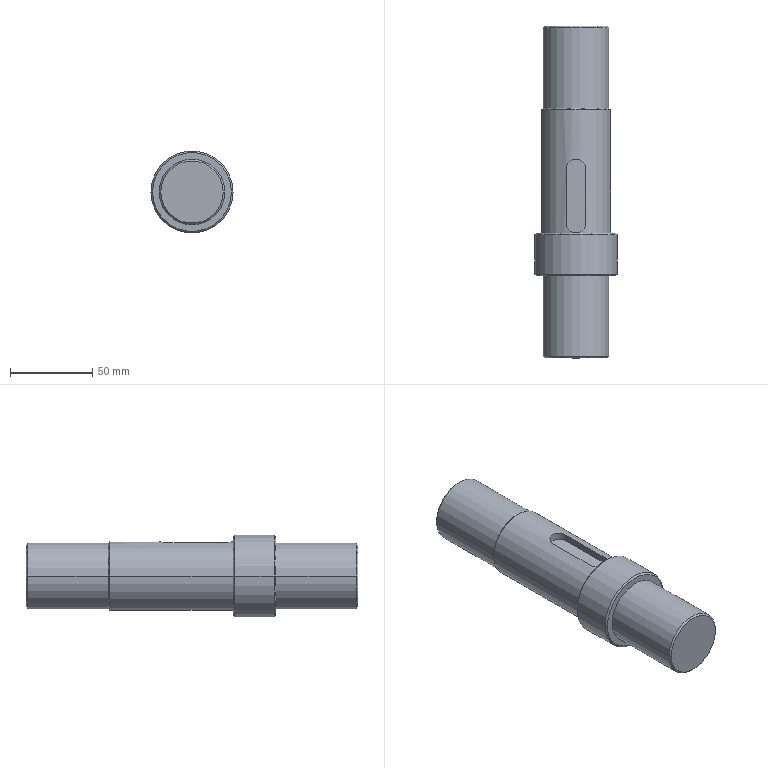Part | SolidWorks | features Chamfer 1, ICE 1, Revolution 1 | 1 solid | 27 faces | box 50 x 202 x 50 mm | volume 279258 mm3 | cone 10 | cylinder 10 | plane 7 | commonest cylinder face diameters 40 x4 12 x2 42 x2 50 x2
STEP:
#1=CARTESIAN_POINT('',(19.,0.,0.));
#2=VERTEX_POINT('',#1);
#3=CARTESIAN_POINT('',(-19.,0.,0.));
#4=VERTEX_POINT('',#3);
#5=CARTESIAN_POINT('',(0.,0.,0.));
#6=DIRECTION('',(0.,-1.,0.));
#7=DIRECTION('',(-1.,0.,0.));
#8=AXIS2_PLACEMENT_3D('',#5,#6,#7);
#9=CIRCLE('',#8,19.);
#10=EDGE_CURVE('',#2,#4,#9,.T.);
#11=ORIENTED_EDGE('',*,*,#10,.F.);
#12=CARTESIAN_POINT('',(20.,1.,0.));
#13=VERTEX_POINT('',#12);
#14=CARTESIAN_POINT('',(20.,1.,0.));
#15=DIRECTION('',(0.7071,0.7071,0.));
#16=VECTOR('',#15,1000.);
#17=LINE('',#14,#16);
#18=EDGE_CURVE('',#2,#13,#17,.T.);
#19=ORIENTED_EDGE('',*,*,#18,.T.);
#20=CARTESIAN_POINT('',(-20.,1.,0.));
#21=VERTEX_POINT('',#20);
#22=CARTESIAN_POINT('',(0.,1.,0.));
#23=DIRECTION('',(0.,1.,0.));
#24=DIRECTION('',(-1.,0.,0.));
#25=AXIS2_PLACEMENT_3D('',#22,#23,#24);
#26=CIRCLE('',#25,20.);
#27=EDGE_CURVE('',#21,#13,#26,.T.);
#28=ORIENTED_EDGE('',*,*,#27,.F.);
#29=CARTESIAN_POINT('',(-20.,1.,0.));
#30=DIRECTION('',(-0.7071,0.7071,0.));
#31=VECTOR('',#30,1000.);
#32=LINE('',#29,#31);
#33=EDGE_CURVE('',#4,#21,#32,.T.);
#34=ORIENTED_EDGE('',*,*,#33,.F.);
#35=EDGE_LOOP('',(#11,#19,#28,#34));
#36=FACE_OUTER_BOUND('',#35,.T.);
#37=CARTESIAN_POINT('',(0.,1.,0.));
#38=DIRECTION('',(0.,1.,0.));
#39=DIRECTION('',(-1.,0.,0.));
#40=AXIS2_PLACEMENT_3D('',#37,#38,#39);
#41=CONICAL_SURFACE('',#40,20.,0.7854);
#42=ADVANCED_FACE('',(#36),#41,.T.);
#43=CARTESIAN_POINT('',(-20.,152.,0.));
#44=VERTEX_POINT('',#43);
#45=CARTESIAN_POINT('',(20.,152.,0.));
#46=VERTEX_POINT('',#45);
#47=CARTESIAN_POINT('',(0.,152.,0.));
#48=DIRECTION('',(0.,1.,0.));
#49=DIRECTION('',(-1.,0.,0.));
#50=AXIS2_PLACEMENT_3D('',#47,#48,#49);
#51=CIRCLE('',#50,20.);
#52=EDGE_CURVE('',#44,#46,#51,.T.);
#53=ORIENTED_EDGE('',*,*,#52,.F.);
#54=CARTESIAN_POINT('',(-21.,151.,0.));
#55=VERTEX_POINT('',#54);
#56=CARTESIAN_POINT('',(-20.,152.,0.));
#57=DIRECTION('',(-0.7071,-0.7071,0.));
#58=VECTOR('',#57,1000.);
#59=LINE('',#56,#58);
#60=EDGE_CURVE('',#44,#55,#59,.T.);
#61=ORIENTED_EDGE('',*,*,#60,.T.);
#62=CARTESIAN_POINT('',(21.,151.,0.));
#63=VERTEX_POINT('',#62);
#64=CARTESIAN_POINT('',(0.,151.,0.));
#65=DIRECTION('',(0.,-1.,0.));
#66=DIRECTION('',(1.,0.,0.));
#67=AXIS2_PLACEMENT_3D('',#64,#65,#66);
#68=CIRCLE('',#67,21.);
#69=EDGE_CURVE('',#63,#55,#68,.T.);
#70=ORIENTED_EDGE('',*,*,#69,.F.);
#71=CARTESIAN_POINT('',(20.,152.,0.));
#72=DIRECTION('',(0.7071,-0.7071,0.));
#73=VECTOR('',#72,1000.);
#74=LINE('',#71,#73);
#75=EDGE_CURVE('',#46,#63,#74,.T.);
#76=ORIENTED_EDGE('',*,*,#75,.F.);
#77=EDGE_LOOP('',(#53,#61,#70,#76));
#78=FACE_OUTER_BOUND('',#77,.T.);
#79=CARTESIAN_POINT('',(0.,152.,0.));
#80=DIRECTION('',(0.,-1.,0.));
#81=DIRECTION('',(1.,0.,0.));
#82=AXIS2_PLACEMENT_3D('',#79,#80,#81);
#83=CONICAL_SURFACE('',#82,20.,0.7854);
#84=ADVANCED_FACE('',(#78),#83,.T.);
#85=CARTESIAN_POINT('',(-19.,202.,0.));
#86=VERTEX_POINT('',#85);
#87=CARTESIAN_POINT('',(19.,202.,0.));
#88=VERTEX_POINT('',#87);
#89=CARTESIAN_POINT('',(0.,202.,0.));
#90=DIRECTION('',(0.,1.,0.));
#91=DIRECTION('',(1.,0.,0.));
#92=AXIS2_PLACEMENT_3D('',#89,#90,#91);
#93=CIRCLE('',#92,19.);
#94=EDGE_CURVE('',#86,#88,#93,.T.);
#95=ORIENTED_EDGE('',*,*,#94,.F.);
#96=CARTESIAN_POINT('',(-20.,201.,0.));
#97=VERTEX_POINT('',#96);
#98=CARTESIAN_POINT('',(-19.,202.,0.));
#99=DIRECTION('',(-0.7071,-0.7071,0.));
#100=VECTOR('',#99,1000.);
#101=LINE('',#98,#100);
#102=EDGE_CURVE('',#86,#97,#101,.T.);
#103=ORIENTED_EDGE('',*,*,#102,.T.);
#104=CARTESIAN_POINT('',(20.,201.,0.));
#105=VERTEX_POINT('',#104);
#106=CARTESIAN_POINT('',(0.,201.,0.));
#107=DIRECTION('',(0.,-1.,0.));
#108=DIRECTION('',(1.,0.,0.));
#109=AXIS2_PLACEMENT_3D('',#106,#107,#108);
#110=CIRCLE('',#109,20.);
#111=EDGE_CURVE('',#105,#97,#110,.T.);
#112=ORIENTED_EDGE('',*,*,#111,.F.);
#113=CARTESIAN_POINT('',(19.,202.,0.));
#114=DIRECTION('',(0.7071,-0.7071,0.));
#115=VECTOR('',#114,1000.);
#116=LINE('',#113,#115);
#117=EDGE_CURVE('',#88,#105,#116,.T.);
#118=ORIENTED_EDGE('',*,*,#117,.F.);
#119=EDGE_LOOP('',(#95,#103,#112,#118));
#120=FACE_OUTER_BOUND('',#119,.T.);
#121=CARTESIAN_POINT('',(0.,202.,0.));
#122=DIRECTION('',(0.,-1.,0.));
#123=DIRECTION('',(1.,0.,0.));
#124=AXIS2_PLACEMENT_3D('',#121,#122,#123);
#125=CONICAL_SURFACE('',#124,19.,0.7854);
#126=ADVANCED_FACE('',(#120),#125,.T.);
#127=CARTESIAN_POINT('',(-24.,76.,0.));
#128=VERTEX_POINT('',#127);
#129=CARTESIAN_POINT('',(24.,76.,0.));
#130=VERTEX_POINT('',#129);
#131=CARTESIAN_POINT('',(0.,76.,0.));
#132=DIRECTION('',(0.,1.,0.));
#133=DIRECTION('',(1.,0.,0.));
#134=AXIS2_PLACEMENT_3D('',#131,#132,#133);
#135=CIRCLE('',#134,24.);
#136=EDGE_CURVE('',#128,#130,#135,.T.);
#137=ORIENTED_EDGE('',*,*,#136,.F.);
#138=CARTESIAN_POINT('',(-25.,75.,0.));
#139=VERTEX_POINT('',#138);
#140=CARTESIAN_POINT('',(-24.,76.,0.));
#141=DIRECTION('',(-0.7071,-0.7071,0.));
#142=VECTOR('',#141,1000.);
#143=LINE('',#140,#142);
#144=EDGE_CURVE('',#128,#139,#143,.T.);
#145=ORIENTED_EDGE('',*,*,#144,.T.);
#146=CARTESIAN_POINT('',(25.,75.,0.));
#147=VERTEX_POINT('',#146);
#148=CARTESIAN_POINT('',(0.,75.,0.));
#149=DIRECTION('',(0.,-1.,0.));
#150=DIRECTION('',(1.,0.,0.));
#151=AXIS2_PLACEMENT_3D('',#148,#149,#150);
#152=CIRCLE('',#151,25.);
#153=EDGE_CURVE('',#147,#139,#152,.T.);
#154=ORIENTED_EDGE('',*,*,#153,.F.);
#155=CARTESIAN_POINT('',(24.,76.,0.));
#156=DIRECTION('',(0.7071,-0.7071,0.));
#157=VECTOR('',#156,1000.);
#158=LINE('',#155,#157);
#159=EDGE_CURVE('',#130,#147,#158,.T.);
#160=ORIENTED_EDGE('',*,*,#159,.F.);
#161=EDGE_LOOP('',(#137,#145,#154,#160));
#162=FACE_OUTER_BOUND('',#161,.T.);
#163=CARTESIAN_POINT('',(0.,76.,0.));
#164=DIRECTION('',(0.,-1.,0.));
#165=DIRECTION('',(1.,0.,0.));
#166=AXIS2_PLACEMENT_3D('',#163,#164,#165);
#167=CONICAL_SURFACE('',#166,24.,0.7854);
#168=ADVANCED_FACE('',(#162),#167,.T.);
#169=CARTESIAN_POINT('',(24.,50.,0.));
#170=VERTEX_POINT('',#169);
#171=CARTESIAN_POINT('',(-24.,50.,0.));
#172=VERTEX_POINT('',#171);
#173=CARTESIAN_POINT('',(0.,50.,0.));
#174=DIRECTION('',(0.,-1.,0.));
#175=DIRECTION('',(-1.,0.,0.));
#176=AXIS2_PLACEMENT_3D('',#173,#174,#175);
#177=CIRCLE('',#176,24.);
#178=EDGE_CURVE('',#170,#172,#177,.T.);
#179=ORIENTED_EDGE('',*,*,#178,.F.);
#180=CARTESIAN_POINT('',(25.,51.,0.));
#181=VERTEX_POINT('',#180);
#182=CARTESIAN_POINT('',(25.,51.,0.));
#183=DIRECTION('',(0.7071,0.7071,0.));
#184=VECTOR('',#183,1000.);
#185=LINE('',#182,#184);
#186=EDGE_CURVE('',#170,#181,#185,.T.);
#187=ORIENTED_EDGE('',*,*,#186,.T.);
#188=CARTESIAN_POINT('',(-25.,51.,0.));
#189=VERTEX_POINT('',#188);
#190=CARTESIAN_POINT('',(0.,51.,0.));
#191=DIRECTION('',(0.,1.,0.));
#192=DIRECTION('',(-1.,0.,0.));
#193=AXIS2_PLACEMENT_3D('',#190,#191,#192);
#194=CIRCLE('',#193,25.);
#195=EDGE_CURVE('',#189,#181,#194,.T.);
#196=ORIENTED_EDGE('',*,*,#195,.F.);
#197=CARTESIAN_POINT('',(-25.,51.,0.));
#198=DIRECTION('',(-0.7071,0.7071,0.));
#199=VECTOR('',#198,1000.);
#200=LINE('',#197,#199);
#201=EDGE_CURVE('',#172,#189,#200,.T.);
#202=ORIENTED_EDGE('',*,*,#201,.F.);
#203=EDGE_LOOP('',(#179,#187,#196,#202));
#204=FACE_OUTER_BOUND('',#203,.T.);
#205=CARTESIAN_POINT('',(0.,51.,0.));
#206=DIRECTION('',(0.,1.,0.));
#207=DIRECTION('',(-1.,0.,0.));
#208=AXIS2_PLACEMENT_3D('',#205,#206,#207);
#209=CONICAL_SURFACE('',#208,25.,0.7854);
#210=ADVANCED_FACE('',(#204),#209,.T.);
#211=ORIENTED_EDGE('',*,*,#52,.T.);
#212=CARTESIAN_POINT('',(20.,202.,0.));
#213=DIRECTION('',(0.,1.,0.));
#214=VECTOR('',#213,1000.);
#215=LINE('',#212,#214);
#216=EDGE_CURVE('',#46,#105,#215,.T.);
#217=ORIENTED_EDGE('',*,*,#216,.T.);
#218=ORIENTED_EDGE('',*,*,#111,.T.);
#219=CARTESIAN_POINT('',(-20.,202.,0.));
#220=DIRECTION('',(0.,1.,0.));
#221=VECTOR('',#220,1000.);
#222=LINE('',#219,#221);
#223=EDGE_CURVE('',#44,#97,#222,.T.);
#224=ORIENTED_EDGE('',*,*,#223,.F.);
#225=EDGE_LOOP('',(#211,#217,#218,#224));
#226=FACE_OUTER_BOUND('',#225,.T.);
#227=CARTESIAN_POINT('',(0.,202.,0.));
#228=DIRECTION('',(0.,1.,0.));
#229=DIRECTION('',(-1.,0.,0.));
#230=AXIS2_PLACEMENT_3D('',#227,#228,#229);
#231=CYLINDRICAL_SURFACE('',#230,20.);
#232=ADVANCED_FACE('',(#226),#231,.T.);
#233=ORIENTED_EDGE('',*,*,#195,.T.);
#234=CARTESIAN_POINT('',(25.,202.,0.));
#235=DIRECTION('',(0.,1.,0.));
#236=VECTOR('',#235,1000.);
#237=LINE('',#234,#236);
#238=EDGE_CURVE('',#181,#147,#237,.T.);
#239=ORIENTED_EDGE('',*,*,#238,.T.);
#240=ORIENTED_EDGE('',*,*,#153,.T.);
#241=CARTESIAN_POINT('',(-25.,202.,0.));
#242=DIRECTION('',(0.,1.,0.));
#243=VECTOR('',#242,1000.);
#244=LINE('',#241,#243);
#245=EDGE_CURVE('',#189,#139,#244,.T.);
#246=ORIENTED_EDGE('',*,*,#245,.F.);
#247=EDGE_LOOP('',(#233,#239,#240,#246));
#248=FACE_OUTER_BOUND('',#247,.T.);
#249=CARTESIAN_POINT('',(0.,202.,0.));
#250=DIRECTION('',(0.,1.,0.));
#251=DIRECTION('',(-1.,0.,0.));
#252=AXIS2_PLACEMENT_3D('',#249,#250,#251);
#253=CYLINDRICAL_SURFACE('',#252,25.);
#254=ADVANCED_FACE('',(#248),#253,.T.);
#255=ORIENTED_EDGE('',*,*,#27,.T.);
#256=CARTESIAN_POINT('',(20.,50.,0.));
#257=VERTEX_POINT('',#256);
#258=CARTESIAN_POINT('',(20.,202.,0.));
#259=DIRECTION('',(0.,1.,0.));
#260=VECTOR('',#259,1000.);
#261=LINE('',#258,#260);
#262=EDGE_CURVE('',#13,#257,#261,.T.);
#263=ORIENTED_EDGE('',*,*,#262,.T.);
#264=CARTESIAN_POINT('',(-20.,50.,0.));
#265=VERTEX_POINT('',#264);
#266=CARTESIAN_POINT('',(0.,50.,0.));
#267=DIRECTION('',(0.,1.,0.));
#268=DIRECTION('',(-1.,0.,0.));
#269=AXIS2_PLACEMENT_3D('',#266,#267,#268);
#270=CIRCLE('',#269,20.);
#271=EDGE_CURVE('',#265,#257,#270,.T.);
#272=ORIENTED_EDGE('',*,*,#271,.F.);
#273=CARTESIAN_POINT('',(-20.,202.,0.));
#274=DIRECTION('',(0.,1.,0.));
#275=VECTOR('',#274,1000.);
#276=LINE('',#273,#275);
#277=EDGE_CURVE('',#21,#265,#276,.T.);
#278=ORIENTED_EDGE('',*,*,#277,.F.);
#279=EDGE_LOOP('',(#255,#263,#272,#278));
#280=FACE_OUTER_BOUND('',#279,.T.);
#281=CARTESIAN_POINT('',(0.,202.,0.));
#282=DIRECTION('',(0.,1.,0.));
#283=DIRECTION('',(-1.,0.,0.));
#284=AXIS2_PLACEMENT_3D('',#281,#282,#283);
#285=CYLINDRICAL_SURFACE('',#284,20.);
#286=ADVANCED_FACE('',(#280),#285,.T.);
#287=CARTESIAN_POINT('',(-6.,82.01,20.125));
#288=VERTEX_POINT('',#287);
#289=CARTESIAN_POINT('',(6.,82.01,20.125));
#290=VERTEX_POINT('',#289);
#291=CARTESIAN_POINT('',(-6.,82.01,20.125));
#292=CARTESIAN_POINT('',(-6.,81.611,20.125));
#293=CARTESIAN_POINT('',(-5.961,81.22,20.136));
#294=CARTESIAN_POINT('',(-5.845,80.643,20.17));
#295=CARTESIAN_POINT('',(-5.798,80.452,20.184));
#296=CARTESIAN_POINT('',(-5.683,80.074,20.217));
#297=CARTESIAN_POINT('',(-5.615,79.887,20.235));
#298=CARTESIAN_POINT('',(-5.389,79.343,20.297));
#299=CARTESIAN_POINT('',(-5.205,78.999,20.346));
#300=CARTESIAN_POINT('',(-4.878,78.512,20.426));
#301=CARTESIAN_POINT('',(-4.761,78.353,20.454));
#302=CARTESIAN_POINT('',(-4.511,78.05,20.51));
#303=CARTESIAN_POINT('',(-4.38,77.905,20.539));
#304=CARTESIAN_POINT('',(-3.968,77.492,20.624));
#305=CARTESIAN_POINT('',(-3.667,77.245,20.68));
#306=CARTESIAN_POINT('',(-3.012,76.806,20.785));
#307=CARTESIAN_POINT('',(-2.666,76.621,20.833));
#308=CARTESIAN_POINT('',(-2.126,76.396,20.893));
#309=CARTESIAN_POINT('',(-1.942,76.329,20.911));
#310=CARTESIAN_POINT('',(-1.565,76.214,20.942));
#311=CARTESIAN_POINT('',(-1.371,76.165,20.956));
#312=CARTESIAN_POINT('',(-0.7899,76.049,20.989));
#313=CARTESIAN_POINT('',(-0.3993,76.01,21.));
#314=CARTESIAN_POINT('',(0.3878,76.01,21.));
#315=CARTESIAN_POINT('',(0.7877,76.049,20.989));
#316=CARTESIAN_POINT('',(1.559,76.203,20.946));
#317=CARTESIAN_POINT('',(1.934,76.317,20.914));
#318=CARTESIAN_POINT('',(2.481,76.543,20.854));
#319=CARTESIAN_POINT('',(2.66,76.628,20.832));
#320=CARTESIAN_POINT('',(3.006,76.813,20.785));
#321=CARTESIAN_POINT('',(3.173,76.914,20.76));
#322=CARTESIAN_POINT('',(3.497,77.13,20.707));
#323=CARTESIAN_POINT('',(3.653,77.247,20.68));
#324=CARTESIAN_POINT('',(3.956,77.495,20.625));
#325=CARTESIAN_POINT('',(4.103,77.627,20.596));
#326=CARTESIAN_POINT('',(4.518,78.043,20.51));
#327=CARTESIAN_POINT('',(4.765,78.343,20.453));
#328=CARTESIAN_POINT('',(5.2,78.991,20.347));
#329=CARTESIAN_POINT('',(5.389,79.342,20.297));
#330=CARTESIAN_POINT('',(5.69,80.065,20.215));
#331=CARTESIAN_POINT('',(5.804,80.439,20.182));
#332=CARTESIAN_POINT('',(5.96,81.213,20.137));
#333=CARTESIAN_POINT('',(6.,81.611,20.125));
#334=CARTESIAN_POINT('',(6.,82.01,20.125));
#335=B_SPLINE_CURVE_WITH_KNOTS('',3,(#291,#292,#293,#294,#295,#296,#297,#298,#299,#300,#301,#302,#303,#304,#305,#306,#307,#308,#309,#310,#311,#312,#313,#314,#315,#316,#317,#318,#319,#320,#321,#322,#323,#324,#325,#326,#327,#328,#329,#330,#331,#332,#333,#334),.UNSPECIFIED.,.F.,.F.,(4,2,2,2,2,2,2,2,2,2,2,2,2,2,2,2,2,2,2,2,2,4),(0.,0.001178,0.001767,0.002356,0.003535,0.004124,0.004713,0.005891,0.007069,0.007658,0.008247,0.009425,0.0106,0.01178,0.01237,0.01296,0.01355,0.01414,0.01532,0.01649,0.01767,0.01885),.UNSPECIFIED.);
#336=EDGE_CURVE('',#288,#290,#335,.T.);
#337=ORIENTED_EDGE('',*,*,#336,.F.);
#338=CARTESIAN_POINT('',(-6.,115.01,20.125));
#339=VERTEX_POINT('',#338);
#340=CARTESIAN_POINT('',(-6.,202.,20.125));
#341=DIRECTION('',(0.,-1.,0.));
#342=VECTOR('',#341,1000.);
#343=LINE('',#340,#342);
#344=EDGE_CURVE('',#339,#288,#343,.T.);
#345=ORIENTED_EDGE('',*,*,#344,.F.);
#346=CARTESIAN_POINT('',(6.,115.01,20.125));
#347=VERTEX_POINT('',#346);
#348=CARTESIAN_POINT('',(6.,115.01,20.125));
#349=CARTESIAN_POINT('',(6.,115.409,20.125));
#350=CARTESIAN_POINT('',(5.961,115.8,20.136));
#351=CARTESIAN_POINT('',(5.845,116.377,20.17));
#352=CARTESIAN_POINT('',(5.798,116.568,20.184));
#353=CARTESIAN_POINT('',(5.683,116.946,20.217));
#354=CARTESIAN_POINT('',(5.615,117.133,20.235));
#355=CARTESIAN_POINT('',(5.389,117.677,20.297));
#356=CARTESIAN_POINT('',(5.205,118.021,20.346));
#357=CARTESIAN_POINT('',(4.878,118.508,20.426));
#358=CARTESIAN_POINT('',(4.761,118.667,20.454));
#359=CARTESIAN_POINT('',(4.511,118.97,20.51));
#360=CARTESIAN_POINT('',(4.38,119.115,20.539));
#361=CARTESIAN_POINT('',(3.968,119.528,20.624));
#362=CARTESIAN_POINT('',(3.667,119.775,20.68));
#363=CARTESIAN_POINT('',(3.012,120.214,20.785));
#364=CARTESIAN_POINT('',(2.666,120.399,20.833));
#365=CARTESIAN_POINT('',(2.126,120.624,20.893));
#366=CARTESIAN_POINT('',(1.942,120.691,20.911));
#367=CARTESIAN_POINT('',(1.565,120.806,20.942));
#368=CARTESIAN_POINT('',(1.371,120.855,20.956));
#369=CARTESIAN_POINT('',(0.7899,120.971,20.989));
#370=CARTESIAN_POINT('',(0.3993,121.01,21.));
#371=CARTESIAN_POINT('',(-0.3878,121.01,21.));
#372=CARTESIAN_POINT('',(-0.7877,120.971,20.989));
#373=CARTESIAN_POINT('',(-1.559,120.817,20.946));
#374=CARTESIAN_POINT('',(-1.934,120.703,20.914));
#375=CARTESIAN_POINT('',(-2.481,120.477,20.854));
#376=CARTESIAN_POINT('',(-2.66,120.392,20.832));
#377=CARTESIAN_POINT('',(-3.006,120.207,20.785));
#378=CARTESIAN_POINT('',(-3.173,120.106,20.76));
#379=CARTESIAN_POINT('',(-3.497,119.89,20.707));
#380=CARTESIAN_POINT('',(-3.653,119.773,20.68));
#381=CARTESIAN_POINT('',(-3.956,119.525,20.625));
#382=CARTESIAN_POINT('',(-4.103,119.393,20.596));
#383=CARTESIAN_POINT('',(-4.518,118.977,20.51));
#384=CARTESIAN_POINT('',(-4.765,118.677,20.453));
#385=CARTESIAN_POINT('',(-5.2,118.029,20.347));
#386=CARTESIAN_POINT('',(-5.389,117.678,20.297));
#387=CARTESIAN_POINT('',(-5.69,116.955,20.215));
#388=CARTESIAN_POINT('',(-5.804,116.581,20.182));
#389=CARTESIAN_POINT('',(-5.96,115.807,20.137));
#390=CARTESIAN_POINT('',(-6.,115.409,20.125));
#391=CARTESIAN_POINT('',(-6.,115.01,20.125));
#392=B_SPLINE_CURVE_WITH_KNOTS('',3,(#348,#349,#350,#351,#352,#353,#354,#355,#356,#357,#358,#359,#360,#361,#362,#363,#364,#365,#366,#367,#368,#369,#370,#371,#372,#373,#374,#375,#376,#377,#378,#379,#380,#381,#382,#383,#384,#385,#386,#387,#388,#389,#390,#391),.UNSPECIFIED.,.F.,.F.,(4,2,2,2,2,2,2,2,2,2,2,2,2,2,2,2,2,2,2,2,2,4),(0.,0.001178,0.001767,0.002356,0.003535,0.004124,0.004713,0.005891,0.007069,0.007658,0.008247,0.009425,0.0106,0.01178,0.01237,0.01296,0.01355,0.01414,0.01532,0.01649,0.01767,0.01885),.UNSPECIFIED.);
#393=EDGE_CURVE('',#347,#339,#392,.T.);
#394=ORIENTED_EDGE('',*,*,#393,.F.);
#395=CARTESIAN_POINT('',(6.,202.,20.125));
#396=DIRECTION('',(0.,1.,0.));
#397=VECTOR('',#396,1000.);
#398=LINE('',#395,#397);
#399=EDGE_CURVE('',#290,#347,#398,.T.);
#400=ORIENTED_EDGE('',*,*,#399,.F.);
#401=EDGE_LOOP('',(#337,#345,#394,#400));
#402=FACE_BOUND('',#401,.T.);
#403=CARTESIAN_POINT('',(-21.,76.,0.));
#404=VERTEX_POINT('',#403);
#405=CARTESIAN_POINT('',(21.,76.,0.));
#406=VERTEX_POINT('',#405);
#407=CARTESIAN_POINT('',(0.,76.,0.));
#408=DIRECTION('',(0.,1.,0.));
#409=DIRECTION('',(-1.,0.,0.));
#410=AXIS2_PLACEMENT_3D('',#407,#408,#409);
#411=CIRCLE('',#410,21.);
#412=EDGE_CURVE('',#404,#406,#411,.T.);
#413=ORIENTED_EDGE('',*,*,#412,.T.);
#414=CARTESIAN_POINT('',(21.,202.,0.));
#415=DIRECTION('',(0.,1.,0.));
#416=VECTOR('',#415,1000.);
#417=LINE('',#414,#416);
#418=EDGE_CURVE('',#406,#63,#417,.T.);
#419=ORIENTED_EDGE('',*,*,#418,.T.);
#420=ORIENTED_EDGE('',*,*,#69,.T.);
#421=CARTESIAN_POINT('',(-21.,202.,0.));
#422=DIRECTION('',(0.,1.,0.));
#423=VECTOR('',#422,1000.);
#424=LINE('',#421,#423);
#425=EDGE_CURVE('',#404,#55,#424,.T.);
#426=ORIENTED_EDGE('',*,*,#425,.F.);
#427=EDGE_LOOP('',(#413,#419,#420,#426));
#428=FACE_OUTER_BOUND('',#427,.T.);
#429=CARTESIAN_POINT('',(0.,202.,0.));
#430=DIRECTION('',(0.,1.,0.));
#431=DIRECTION('',(-1.,0.,0.));
#432=AXIS2_PLACEMENT_3D('',#429,#430,#431);
#433=CYLINDRICAL_SURFACE('',#432,21.);
#434=ADVANCED_FACE('',(#402,#428),#433,.T.);
#435=ORIENTED_EDGE('',*,*,#418,.F.);
#436=CARTESIAN_POINT('',(0.,76.,0.));
#437=DIRECTION('',(0.,1.,0.));
#438=DIRECTION('',(-1.,0.,0.));
#439=AXIS2_PLACEMENT_3D('',#436,#437,#438);
#440=CIRCLE('',#439,21.);
#441=EDGE_CURVE('',#406,#404,#440,.T.);
#442=ORIENTED_EDGE('',*,*,#441,.T.);
#443=ORIENTED_EDGE('',*,*,#425,.T.);
#444=CARTESIAN_POINT('',(0.,151.,0.));
#445=DIRECTION('',(0.,-1.,0.));
#446=DIRECTION('',(1.,0.,0.));
#447=AXIS2_PLACEMENT_3D('',#444,#445,#446);
#448=CIRCLE('',#447,21.);
#449=EDGE_CURVE('',#55,#63,#448,.T.);
#450=ORIENTED_EDGE('',*,*,#449,.T.);
#451=EDGE_LOOP('',(#435,#442,#443,#450));
#452=FACE_OUTER_BOUND('',#451,.T.);
#453=CARTESIAN_POINT('',(0.,202.,0.));
#454=DIRECTION('',(0.,1.,0.));
#455=DIRECTION('',(-1.,0.,0.));
#456=AXIS2_PLACEMENT_3D('',#453,#454,#455);
#457=CYLINDRICAL_SURFACE('',#456,21.);
#458=ADVANCED_FACE('',(#452),#457,.T.);
#459=CARTESIAN_POINT('',(0.,0.,0.));
#460=DIRECTION('',(0.,-1.,0.));
#461=DIRECTION('',(-1.,0.,0.));
#462=AXIS2_PLACEMENT_3D('',#459,#460,#461);
#463=CIRCLE('',#462,19.);
#464=EDGE_CURVE('',#4,#2,#463,.T.);
#465=ORIENTED_EDGE('',*,*,#464,.T.);
#466=ORIENTED_EDGE('',*,*,#10,.T.);
#467=EDGE_LOOP('',(#465,#466));
#468=FACE_OUTER_BOUND('',#467,.T.);
#469=CARTESIAN_POINT('',(0.,0.,0.));
#470=DIRECTION('',(0.,1.,0.));
#471=DIRECTION('',(-1.,0.,0.));
#472=AXIS2_PLACEMENT_3D('',#469,#470,#471);
#473=PLANE('',#472);
#474=ADVANCED_FACE('',(#468),#473,.F.);
#475=ORIENTED_EDGE('',*,*,#262,.F.);
#476=CARTESIAN_POINT('',(0.,1.,0.));
#477=DIRECTION('',(0.,1.,0.));
#478=DIRECTION('',(-1.,0.,0.));
#479=AXIS2_PLACEMENT_3D('',#476,#477,#478);
#480=CIRCLE('',#479,20.);
#481=EDGE_CURVE('',#13,#21,#480,.T.);
#482=ORIENTED_EDGE('',*,*,#481,.T.);
#483=ORIENTED_EDGE('',*,*,#277,.T.);
#484=CARTESIAN_POINT('',(0.,50.,0.));
#485=DIRECTION('',(0.,1.,0.));
#486=DIRECTION('',(-1.,0.,0.));
#487=AXIS2_PLACEMENT_3D('',#484,#485,#486);
#488=CIRCLE('',#487,20.);
#489=EDGE_CURVE('',#257,#265,#488,.T.);
#490=ORIENTED_EDGE('',*,*,#489,.F.);
#491=EDGE_LOOP('',(#475,#482,#483,#490));
#492=FACE_OUTER_BOUND('',#491,.T.);
#493=CARTESIAN_POINT('',(0.,202.,0.));
#494=DIRECTION('',(0.,1.,0.));
#495=DIRECTION('',(-1.,0.,0.));
#496=AXIS2_PLACEMENT_3D('',#493,#494,#495);
#497=CYLINDRICAL_SURFACE('',#496,20.);
#498=ADVANCED_FACE('',(#492),#497,.T.);
#499=CARTESIAN_POINT('',(0.,50.,0.));
#500=DIRECTION('',(0.,-1.,0.));
#501=DIRECTION('',(-1.,0.,0.));
#502=AXIS2_PLACEMENT_3D('',#499,#500,#501);
#503=CIRCLE('',#502,24.);
#504=EDGE_CURVE('',#172,#170,#503,.T.);
#505=ORIENTED_EDGE('',*,*,#504,.T.);
#506=ORIENTED_EDGE('',*,*,#178,.T.);
#507=EDGE_LOOP('',(#505,#506));
#508=FACE_OUTER_BOUND('',#507,.T.);
#509=ORIENTED_EDGE('',*,*,#271,.T.);
#510=ORIENTED_EDGE('',*,*,#489,.T.);
#511=EDGE_LOOP('',(#509,#510));
#512=FACE_BOUND('',#511,.T.);
#513=CARTESIAN_POINT('',(20.,50.,0.));
#514=DIRECTION('',(0.,1.,0.));
#515=DIRECTION('',(-1.,0.,0.));
#516=AXIS2_PLACEMENT_3D('',#513,#514,#515);
#517=PLANE('',#516);
#518=ADVANCED_FACE('',(#508,#512),#517,.F.);
#519=ORIENTED_EDGE('',*,*,#238,.F.);
#520=CARTESIAN_POINT('',(0.,51.,0.));
#521=DIRECTION('',(0.,1.,0.));
#522=DIRECTION('',(-1.,0.,0.));
#523=AXIS2_PLACEMENT_3D('',#520,#521,#522);
#524=CIRCLE('',#523,25.);
#525=EDGE_CURVE('',#181,#189,#524,.T.);
#526=ORIENTED_EDGE('',*,*,#525,.T.);
#527=ORIENTED_EDGE('',*,*,#245,.T.);
#528=CARTESIAN_POINT('',(0.,75.,0.));
#529=DIRECTION('',(0.,-1.,0.));
#530=DIRECTION('',(1.,0.,0.));
#531=AXIS2_PLACEMENT_3D('',#528,#529,#530);
#532=CIRCLE('',#531,25.);
#533=EDGE_CURVE('',#139,#147,#532,.T.);
#534=ORIENTED_EDGE('',*,*,#533,.T.);
#535=EDGE_LOOP('',(#519,#526,#527,#534));
#536=FACE_OUTER_BOUND('',#535,.T.);
#537=CARTESIAN_POINT('',(0.,202.,0.));
#538=DIRECTION('',(0.,1.,0.));
#539=DIRECTION('',(-1.,0.,0.));
#540=AXIS2_PLACEMENT_3D('',#537,#538,#539);
#541=CYLINDRICAL_SURFACE('',#540,25.);
#542=ADVANCED_FACE('',(#536),#541,.T.);
#543=CARTESIAN_POINT('',(0.,76.,0.));
#544=DIRECTION('',(0.,1.,0.));
#545=DIRECTION('',(1.,0.,0.));
#546=AXIS2_PLACEMENT_3D('',#543,#544,#545);
#547=CIRCLE('',#546,24.);
#548=EDGE_CURVE('',#130,#128,#547,.T.);
#549=ORIENTED_EDGE('',*,*,#548,.T.);
#550=ORIENTED_EDGE('',*,*,#136,.T.);
#551=EDGE_LOOP('',(#549,#550));
#552=FACE_OUTER_BOUND('',#551,.T.);
#553=ORIENTED_EDGE('',*,*,#412,.F.);
#554=ORIENTED_EDGE('',*,*,#441,.F.);
#555=EDGE_LOOP('',(#553,#554));
#556=FACE_BOUND('',#555,.T.);
#557=CARTESIAN_POINT('',(25.,76.,0.));
#558=DIRECTION('',(0.,-1.,0.));
#559=DIRECTION('',(1.,0.,0.));
#560=AXIS2_PLACEMENT_3D('',#557,#558,#559);
#561=PLANE('',#560);
#562=ADVANCED_FACE('',(#552,#556),#561,.F.);
#563=ORIENTED_EDGE('',*,*,#216,.F.);
#564=CARTESIAN_POINT('',(0.,152.,0.));
#565=DIRECTION('',(0.,1.,0.));
#566=DIRECTION('',(-1.,0.,0.));
#567=AXIS2_PLACEMENT_3D('',#564,#565,#566);
#568=CIRCLE('',#567,20.);
#569=EDGE_CURVE('',#46,#44,#568,.T.);
#570=ORIENTED_EDGE('',*,*,#569,.T.);
#571=ORIENTED_EDGE('',*,*,#223,.T.);
#572=CARTESIAN_POINT('',(0.,201.,0.));
#573=DIRECTION('',(0.,-1.,0.));
#574=DIRECTION('',(1.,0.,0.));
#575=AXIS2_PLACEMENT_3D('',#572,#573,#574);
#576=CIRCLE('',#575,20.);
#577=EDGE_CURVE('',#97,#105,#576,.T.);
#578=ORIENTED_EDGE('',*,*,#577,.T.);
#579=EDGE_LOOP('',(#563,#570,#571,#578));
#580=FACE_OUTER_BOUND('',#579,.T.);
#581=CARTESIAN_POINT('',(0.,202.,0.));
#582=DIRECTION('',(0.,1.,0.));
#583=DIRECTION('',(-1.,0.,0.));
#584=AXIS2_PLACEMENT_3D('',#581,#582,#583);
#585=CYLINDRICAL_SURFACE('',#584,20.);
#586=ADVANCED_FACE('',(#580),#585,.T.);
#587=CARTESIAN_POINT('',(0.,202.,0.));
#588=DIRECTION('',(0.,1.,0.));
#589=DIRECTION('',(1.,0.,0.));
#590=AXIS2_PLACEMENT_3D('',#587,#588,#589);
#591=CIRCLE('',#590,19.);
#592=EDGE_CURVE('',#88,#86,#591,.T.);
#593=ORIENTED_EDGE('',*,*,#592,.T.);
#594=ORIENTED_EDGE('',*,*,#94,.T.);
#595=EDGE_LOOP('',(#593,#594));
#596=FACE_OUTER_BOUND('',#595,.T.);
#597=CARTESIAN_POINT('',(20.,202.,0.));
#598=DIRECTION('',(0.,-1.,0.));
#599=DIRECTION('',(1.,0.,0.));
#600=AXIS2_PLACEMENT_3D('',#597,#598,#599);
#601=PLANE('',#600);
#602=ADVANCED_FACE('',(#596),#601,.F.);
#603=ORIENTED_EDGE('',*,*,#186,.F.);
#604=ORIENTED_EDGE('',*,*,#504,.F.);
#605=ORIENTED_EDGE('',*,*,#201,.T.);
#606=ORIENTED_EDGE('',*,*,#525,.F.);
#607=EDGE_LOOP('',(#603,#604,#605,#606));
#608=FACE_OUTER_BOUND('',#607,.T.);
#609=CARTESIAN_POINT('',(0.,51.,0.));
#610=DIRECTION('',(0.,1.,0.));
#611=DIRECTION('',(-1.,0.,0.));
#612=AXIS2_PLACEMENT_3D('',#609,#610,#611);
#613=CONICAL_SURFACE('',#612,25.,0.7854);
#614=ADVANCED_FACE('',(#608),#613,.T.);
#615=ORIENTED_EDGE('',*,*,#144,.F.);
#616=ORIENTED_EDGE('',*,*,#548,.F.);
#617=ORIENTED_EDGE('',*,*,#159,.T.);
#618=ORIENTED_EDGE('',*,*,#533,.F.);
#619=EDGE_LOOP('',(#615,#616,#617,#618));
#620=FACE_OUTER_BOUND('',#619,.T.);
#621=CARTESIAN_POINT('',(0.,76.,0.));
#622=DIRECTION('',(0.,-1.,0.));
#623=DIRECTION('',(1.,0.,0.));
#624=AXIS2_PLACEMENT_3D('',#621,#622,#623);
#625=CONICAL_SURFACE('',#624,24.,0.7854);
#626=ADVANCED_FACE('',(#620),#625,.T.);
#627=ORIENTED_EDGE('',*,*,#102,.F.);
#628=ORIENTED_EDGE('',*,*,#592,.F.);
#629=ORIENTED_EDGE('',*,*,#117,.T.);
#630=ORIENTED_EDGE('',*,*,#577,.F.);
#631=EDGE_LOOP('',(#627,#628,#629,#630));
#632=FACE_OUTER_BOUND('',#631,.T.);
#633=CARTESIAN_POINT('',(0.,202.,0.));
#634=DIRECTION('',(0.,-1.,0.));
#635=DIRECTION('',(1.,0.,0.));
#636=AXIS2_PLACEMENT_3D('',#633,#634,#635);
#637=CONICAL_SURFACE('',#636,19.,0.7854);
#638=ADVANCED_FACE('',(#632),#637,.T.);
#639=ORIENTED_EDGE('',*,*,#60,.F.);
#640=ORIENTED_EDGE('',*,*,#569,.F.);
#641=ORIENTED_EDGE('',*,*,#75,.T.);
#642=ORIENTED_EDGE('',*,*,#449,.F.);
#643=EDGE_LOOP('',(#639,#640,#641,#642));
#644=FACE_OUTER_BOUND('',#643,.T.);
#645=CARTESIAN_POINT('',(0.,152.,0.));
#646=DIRECTION('',(0.,-1.,0.));
#647=DIRECTION('',(1.,0.,0.));
#648=AXIS2_PLACEMENT_3D('',#645,#646,#647);
#649=CONICAL_SURFACE('',#648,20.,0.7854);
#650=ADVANCED_FACE('',(#644),#649,.T.);
#651=ORIENTED_EDGE('',*,*,#18,.F.);
#652=ORIENTED_EDGE('',*,*,#464,.F.);
#653=ORIENTED_EDGE('',*,*,#33,.T.);
#654=ORIENTED_EDGE('',*,*,#481,.F.);
#655=EDGE_LOOP('',(#651,#652,#653,#654));
#656=FACE_OUTER_BOUND('',#655,.T.);
#657=CARTESIAN_POINT('',(0.,1.,0.));
#658=DIRECTION('',(0.,1.,0.));
#659=DIRECTION('',(-1.,0.,0.));
#660=AXIS2_PLACEMENT_3D('',#657,#658,#659);
#661=CONICAL_SURFACE('',#660,20.,0.7854);
#662=ADVANCED_FACE('',(#656),#661,.T.);
#663=ORIENTED_EDGE('',*,*,#336,.T.);
#664=CARTESIAN_POINT('',(6.,82.01,16.));
#665=VERTEX_POINT('',#664);
#666=CARTESIAN_POINT('',(6.,82.01,26.));
#667=DIRECTION('',(0.,0.,-1.));
#668=VECTOR('',#667,1000.);
#669=LINE('',#666,#668);
#670=EDGE_CURVE('',#290,#665,#669,.T.);
#671=ORIENTED_EDGE('',*,*,#670,.T.);
#672=CARTESIAN_POINT('',(-6.,82.01,16.));
#673=VERTEX_POINT('',#672);
#674=CARTESIAN_POINT('',(0.,82.01,16.));
#675=DIRECTION('',(0.,0.,1.));
#676=DIRECTION('',(1.,0.,0.));
#677=AXIS2_PLACEMENT_3D('',#674,#675,#676);
#678=CIRCLE('',#677,6.);
#679=EDGE_CURVE('',#673,#665,#678,.T.);
#680=ORIENTED_EDGE('',*,*,#679,.F.);
#681=CARTESIAN_POINT('',(-6.,82.01,26.));
#682=DIRECTION('',(0.,0.,-1.));
#683=VECTOR('',#682,1000.);
#684=LINE('',#681,#683);
#685=EDGE_CURVE('',#288,#673,#684,.T.);
#686=ORIENTED_EDGE('',*,*,#685,.F.);
#687=EDGE_LOOP('',(#663,#671,#680,#686));
#688=FACE_OUTER_BOUND('',#687,.T.);
#689=CARTESIAN_POINT('',(0.,82.01,26.));
#690=DIRECTION('',(0.,0.,-1.));
#691=DIRECTION('',(-1.,0.,0.));
#692=AXIS2_PLACEMENT_3D('',#689,#690,#691);
#693=CYLINDRICAL_SURFACE('',#692,6.);
#694=ADVANCED_FACE('',(#688),#693,.F.);
#695=ORIENTED_EDGE('',*,*,#399,.T.);
#696=CARTESIAN_POINT('',(6.,115.01,16.));
#697=VERTEX_POINT('',#696);
#698=CARTESIAN_POINT('',(6.,115.01,26.));
#699=DIRECTION('',(0.,0.,-1.));
#700=VECTOR('',#699,1000.);
#701=LINE('',#698,#700);
#702=EDGE_CURVE('',#347,#697,#701,.T.);
#703=ORIENTED_EDGE('',*,*,#702,.T.);
#704=CARTESIAN_POINT('',(6.,82.01,16.));
#705=DIRECTION('',(0.,1.,0.));
#706=VECTOR('',#705,1000.);
#707=LINE('',#704,#706);
#708=EDGE_CURVE('',#665,#697,#707,.T.);
#709=ORIENTED_EDGE('',*,*,#708,.F.);
#710=ORIENTED_EDGE('',*,*,#670,.F.);
#711=EDGE_LOOP('',(#695,#703,#709,#710));
#712=FACE_OUTER_BOUND('',#711,.T.);
#713=CARTESIAN_POINT('',(6.,82.01,26.));
#714=DIRECTION('',(-1.,0.,0.));
#715=DIRECTION('',(0.,-1.,0.));
#716=AXIS2_PLACEMENT_3D('',#713,#714,#715);
#717=PLANE('',#716);
#718=ADVANCED_FACE('',(#712),#717,.T.);
#719=ORIENTED_EDGE('',*,*,#393,.T.);
#720=CARTESIAN_POINT('',(-6.,115.01,16.));
#721=VERTEX_POINT('',#720);
#722=CARTESIAN_POINT('',(-6.,115.01,26.));
#723=DIRECTION('',(0.,0.,-1.));
#724=VECTOR('',#723,1000.);
#725=LINE('',#722,#724);
#726=EDGE_CURVE('',#339,#721,#725,.T.);
#727=ORIENTED_EDGE('',*,*,#726,.T.);
#728=CARTESIAN_POINT('',(0.,115.01,16.));
#729=DIRECTION('',(0.,0.,1.));
#730=DIRECTION('',(1.,0.,0.));
#731=AXIS2_PLACEMENT_3D('',#728,#729,#730);
#732=CIRCLE('',#731,6.);
#733=EDGE_CURVE('',#697,#721,#732,.T.);
#734=ORIENTED_EDGE('',*,*,#733,.F.);
#735=ORIENTED_EDGE('',*,*,#702,.F.);
#736=EDGE_LOOP('',(#719,#727,#734,#735));
#737=FACE_OUTER_BOUND('',#736,.T.);
#738=CARTESIAN_POINT('',(0.,115.01,26.));
#739=DIRECTION('',(0.,0.,-1.));
#740=DIRECTION('',(-1.,0.,0.));
#741=AXIS2_PLACEMENT_3D('',#738,#739,#740);
#742=CYLINDRICAL_SURFACE('',#741,6.);
#743=ADVANCED_FACE('',(#737),#742,.F.);
#744=ORIENTED_EDGE('',*,*,#344,.T.);
#745=ORIENTED_EDGE('',*,*,#685,.T.);
#746=CARTESIAN_POINT('',(-6.,82.01,16.));
#747=DIRECTION('',(0.,-1.,0.));
#748=VECTOR('',#747,1000.);
#749=LINE('',#746,#748);
#750=EDGE_CURVE('',#721,#673,#749,.T.);
#751=ORIENTED_EDGE('',*,*,#750,.F.);
#752=ORIENTED_EDGE('',*,*,#726,.F.);
#753=EDGE_LOOP('',(#744,#745,#751,#752));
#754=FACE_OUTER_BOUND('',#753,.T.);
#755=CARTESIAN_POINT('',(-6.,82.01,26.));
#756=DIRECTION('',(1.,0.,0.));
#757=DIRECTION('',(0.,1.,0.));
#758=AXIS2_PLACEMENT_3D('',#755,#756,#757);
#759=PLANE('',#758);
#760=ADVANCED_FACE('',(#754),#759,.T.);
#761=ORIENTED_EDGE('',*,*,#679,.T.);
#762=ORIENTED_EDGE('',*,*,#708,.T.);
#763=ORIENTED_EDGE('',*,*,#733,.T.);
#764=ORIENTED_EDGE('',*,*,#750,.T.);
#765=EDGE_LOOP('',(#761,#762,#763,#764));
#766=FACE_OUTER_BOUND('',#765,.T.);
#767=CARTESIAN_POINT('',(0.,82.01,16.));
#768=DIRECTION('',(0.,0.,1.));
#769=DIRECTION('',(1.,0.,0.));
#770=AXIS2_PLACEMENT_3D('',#767,#768,#769);
#771=PLANE('',#770);
#772=ADVANCED_FACE('',(#766),#771,.T.);
#773=CLOSED_SHELL('',(#42,#84,#126,#168,#210,#232,#254,#286,#434,#458,#474,#498,#518,#542,#562,#586,#602,#614,#626,#638,#650,#662,#694,#718,#743,#760,#772));
#774=MANIFOLD_SOLID_BREP('',#773);
#775=CARTESIAN_POINT('',(0.,0.,0.));
#776=DIRECTION('',(0.,0.,1.));
#777=DIRECTION('',(1.,0.,0.));
#778=AXIS2_PLACEMENT_3D('',#775,#776,#777);
#779=(LENGTH_UNIT()NAMED_UNIT(*)SI_UNIT(.MILLI.,.METRE.));
#780=UNCERTAINTY_MEASURE_WITH_UNIT(LENGTH_MEASURE(0.00001),#779,'','');
#781=(NAMED_UNIT(*)PLANE_ANGLE_UNIT()SI_UNIT($,.RADIAN.));
#782=(NAMED_UNIT(*)SI_UNIT($,.STERADIAN.)SOLID_ANGLE_UNIT());
#783=(GEOMETRIC_REPRESENTATION_CONTEXT(3)GLOBAL_UNCERTAINTY_ASSIGNED_CONTEXT((#780))GLOBAL_UNIT_ASSIGNED_CONTEXT((#779,#781,#782))REPRESENTATION_CONTEXT('',''));
#784=ADVANCED_BREP_SHAPE_REPRESENTATION('',(#774,#778),#783);